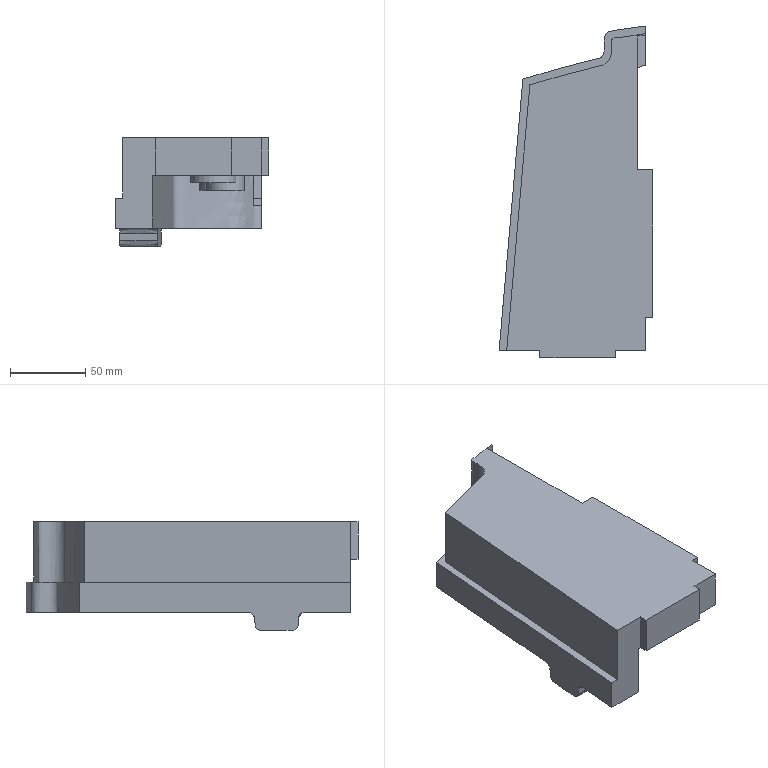Part | NX | features solid 2 | 1 solid | 39 faces | box 102.12 x 220.415 x 72 mm | volume 599805 mm3 | plane 21 | spline 14 | cylinder 4 | commonest cylinder face diameters 25 x2 30 x2